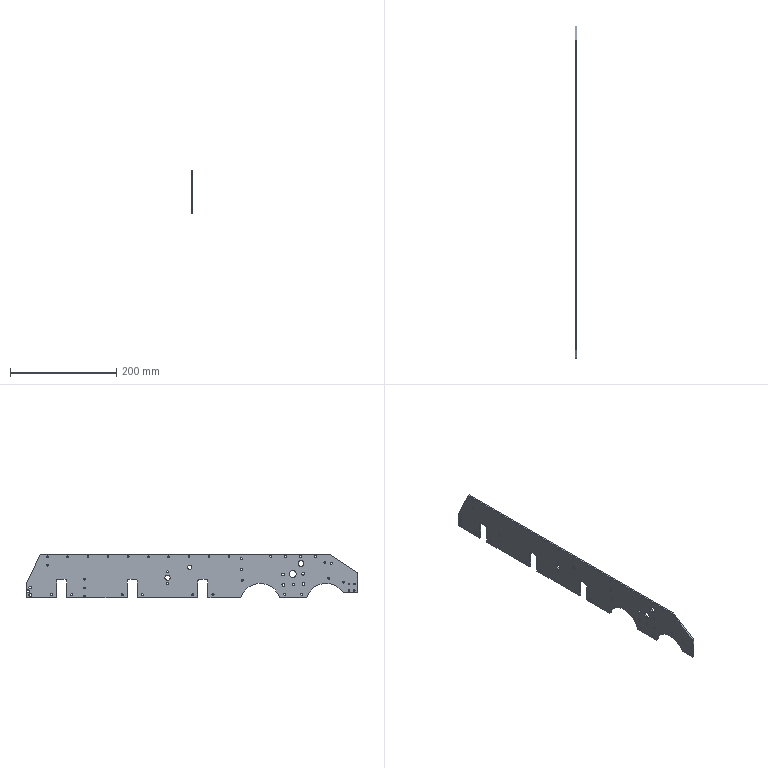Part | STEP file | 1-01.1 | 1 solid | 81 faces | box 3 x 625 x 82.5 mm | volume 131350 mm3 | cylinder 59 | plane 22 | commonest cylinder face diameters 3 x21 4 x17 5 x8 6 x6 76 x2 4.035 x1